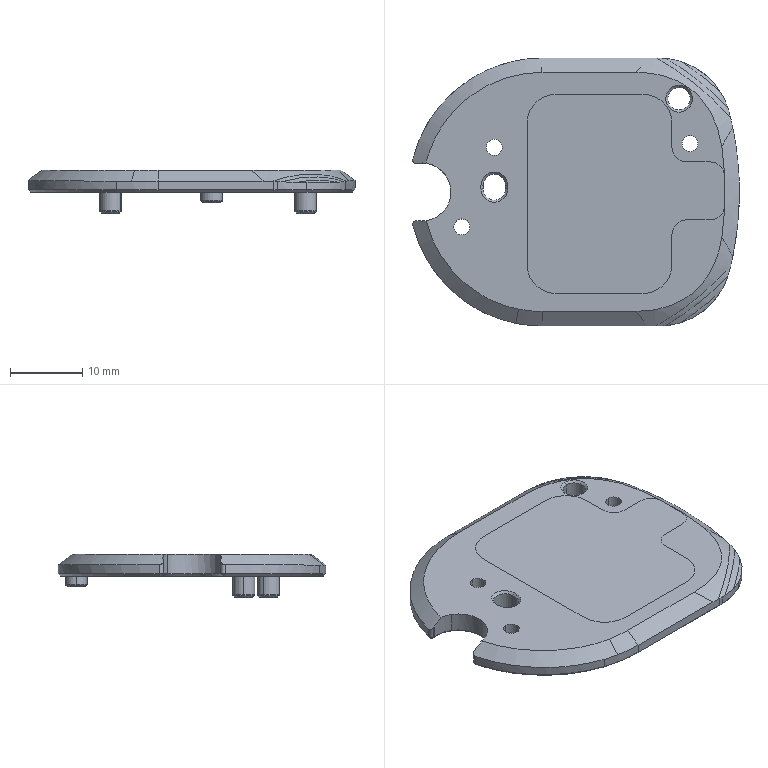NC program | NX | posted with a generic post | part box 45.101 x 36.973 x 6 mm
Lines 4825 to 5084 of 5084:
(PLANAR_MILL_COPY_COPY , TOOL : D6A45)
N9594 T01 M6
N9596 G54
N9598 G17 G0 G90 X-0.654 Y21.303 S9500 M3
N9600 G43 Z30. H1
N9602 Z-1.5
N9604 G94 G1 Z-4.5 F1250.
N9606 X-0.572 Y20.415
N9608 G3 X-0.145 Y19.685 R1.
N9610 G1 X4.605
N9612 G2 X23.698 Y4.829 R19.7
N9614 X21.748 Y2.738 R1.7
N9616 G3 X21.748 Y-2.773 R-2.8
N9618 G2 X23.697 Y-4.864 R1.7
N9620 X10.779 Y-18.722 R19.7
N9622 X7.772 Y-19.444 R19.699
N9624 X4.69 Y-19.686 R19.701
N9626 G1 X-11.31 Y-19.685
N9628 G2 X-11.562 Y-19.683 R19.698
N9630 X-11.814 Y-19.678 R19.699
N9632 X-16.395 Y-18.568 R11.2
N9634 X-22.306 Y-11.325 R11.2
N9636 X-22.304 Y11.3 R45.001
N9638 X-11.747 Y19.68 R11.2
N9640 X-11.247 Y19.686 R19.699
N9642 G1 X-5.267
N9644 G3 X-4.84 Y20.415 R1.
N9646 G1 X-4.757 Y21.303
N9648 Z-1.5
N9650 G0 Z30.
(PLANAR_MILL_COPY_COPY_COPY , TOOL : D6A45)
N9652 X-16.558 Y6.929
N9654 Z-1.
N9656 G1 X-16.576 Y6.442 Z-1.132
N9658 X-16.348 Y6.048 Z-1.254
N9660 X-15.954 Y5.82 Z-1.376
N9662 X-15.498 Z-1.498
N9664 X-15.104 Y6.048 Z-1.62
N9666 X-14.876 Y6.442 Z-1.742
N9668 Y6.898 Z-1.864
N9670 X-15.104 Y7.292 Z-1.986
N9672 X-15.498 Y7.52 Z-2.108
N9674 X-15.954 Z-2.23
N9676 X-16.348 Y7.292 Z-2.352
N9678 X-16.576 Y6.898 Z-2.474
N9680 Y6.442 Z-2.596
N9682 X-16.348 Y6.048 Z-2.718
N9684 X-15.954 Y5.82 Z-2.84
N9686 X-15.498 Z-2.963
N9688 X-15.104 Y6.048 Z-3.085
N9690 X-14.876 Y6.442 Z-3.207
N9692 Y6.898 Z-3.329
N9694 X-15.104 Y7.292 Z-3.451
N9696 X-15.498 Y7.52 Z-3.573
N9698 X-15.954 Z-3.695
N9700 X-16.348 Y7.292 Z-3.817
N9702 X-16.576 Y6.898 Z-3.939
N9704 Y6.67 Z-4.
N9706 G3 X-15.726 Y5.82 R0.85
N9708 X-16.576 Y6.67 R-0.85
N9710 X-16.397 Y6.287 R0.5
N9712 G1 Z-1.
N9714 G0 Z30.
N9716 X-14.764 Y12.485
N9718 Z-1.
N9720 G1 X-14.707 Y12.389 Z-1.03
N9722 X-14.426 Y12.22 Z-1.118
N9724 X-14.026 Z-1.225
N9726 X-13.745 Y12.389 Z-1.313
N9728 X-13.576 Y12.67 Z-1.401
N9730 Y13.07 Z-1.508
N9732 X-13.745 Y13.351 Z-1.596
N9734 X-14.026 Y13.52 Z-1.684
N9736 X-14.426 Z-1.791
N9738 X-14.707 Y13.351 Z-1.879
N9740 X-14.876 Y13.07 Z-1.967
N9742 Y12.67 Z-2.074
N9744 X-14.707 Y12.389 Z-2.161
N9746 X-14.426 Y12.22 Z-2.249
N9748 X-14.026 Z-2.356
N9750 X-13.745 Y12.389 Z-2.444
N9752 X-13.576 Y12.67 Z-2.532
N9754 Y13.07 Z-2.639
N9756 X-13.745 Y13.351 Z-2.727
N9758 X-14.026 Y13.52 Z-2.815
N9760 X-14.426 Z-2.922
N9762 X-14.707 Y13.351 Z-3.01
N9764 X-14.876 Y13.07 Z-3.098
N9766 Y12.67 Z-3.205
N9768 X-14.707 Y12.389 Z-3.293
N9770 X-14.426 Y12.22 Z-3.381
N9772 X-14.026 Z-3.488
N9774 X-13.745 Y12.389 Z-3.576
N9776 X-13.576 Y12.67 Z-3.664
N9778 Y13.07 Z-3.771
N9780 X-13.745 Y13.351 Z-3.859
N9782 X-14.026 Y13.52 Z-3.946
N9784 X-14.226 Z-4.
N9786 G3 X-14.876 Y12.87 R0.65
N9788 X-14.226 Y13.52 R-0.65
N9790 X-14.609 Y13.341 R0.5
N9792 G1 Z-1.
N9794 G0 Z30.
N9796 X12.106 Y5.911
N9798 Z-1.
N9800 G1 X12.124 Y6.398 Z-1.132
N9802 X11.896 Y6.792 Z-1.254
N9804 X11.502 Y7.02 Z-1.376
N9806 X11.046 Z-1.498
N9808 X10.652 Y6.792 Z-1.62
N9810 X10.424 Y6.398 Z-1.742
N9812 Y5.942 Z-1.864
N9814 X10.652 Y5.548 Z-1.986
N9816 X11.046 Y5.32 Z-2.108
N9818 X11.502 Z-2.23
N9820 X11.896 Y5.548 Z-2.352
N9822 X12.124 Y5.942 Z-2.474
N9824 Y6.398 Z-2.596
N9826 X11.896 Y6.792 Z-2.718
N9828 X11.502 Y7.02 Z-2.84
N9830 X11.046 Z-2.963
N9832 X10.652 Y6.792 Z-3.085
N9834 X10.424 Y6.398 Z-3.207
N9836 Y5.942 Z-3.329
N9838 X10.652 Y5.548 Z-3.451
N9840 X11.046 Y5.32 Z-3.573
N9842 X11.502 Z-3.695
N9844 X11.896 Y5.548 Z-3.817
N9846 X12.124 Y5.942 Z-3.939
N9848 Y6.17 Z-4.
N9850 G3 X11.274 Y7.02 R0.85
N9852 X12.124 Y6.17 R-0.85
N9854 X11.946 Y6.553 R0.5
N9856 G1 Z-1.
N9858 G0 Z30.
N9860 X11.769 Y-0.038
N9862 Z-1.
N9864 G1 X11.924 Y0.22 Z-1.081
N9866 Y1.12 Z-1.322
N9868 X11.755 Y1.401 Z-1.41
N9870 X11.474 Y1.57 Z-1.498
N9872 X11.074 Z-1.605
N9874 X10.793 Y1.401 Z-1.693
N9876 X10.624 Y1.12 Z-1.78
N9878 Y0.22 Z-2.021
N9880 X10.793 Y-0.061 Z-2.109
N9882 X11.074 Y-0.23 Z-2.197
N9884 X11.474 Z-2.304
N9886 X11.755 Y-0.061 Z-2.392
N9888 X11.924 Y0.22 Z-2.48
N9890 Y1.12 Z-2.721
N9892 X11.755 Y1.401 Z-2.809
N9894 X11.474 Y1.57 Z-2.897
N9896 X11.074 Z-3.004
N9898 X10.793 Y1.401 Z-3.092
N9900 X10.624 Y1.12 Z-3.18
N9902 Y0.22 Z-3.421
N9904 X10.793 Y-0.061 Z-3.509
N9906 X11.074 Y-0.23 Z-3.597
N9908 X11.474 Z-3.704
N9910 X11.755 Y-0.061 Z-3.792
N9912 X11.924 Y0.22 Z-3.879
N9914 Y0.67 Z-4.
N9916 Y0.92
N9918 G3 X11.274 Y1.57 R0.65
N9920 X10.624 Y0.92 R0.65
N9922 G1 Y0.42
N9924 G3 X11.274 Y-0.23 R0.65
N9926 X11.924 Y0.42 R0.65
N9928 G1 Y0.67
N9930 G3 X11.567 Y1.436 R1.
N9932 G1 Z-1.
N9934 G0 Z30.
N9936 X15.515 Y-5.662
N9938 Z-1.
N9940 G1 X16.002 Y-5.68 Z-1.132
N9942 X16.396 Y-5.452 Z-1.254
N9944 X16.624 Y-5.058 Z-1.376
N9946 Y-4.602 Z-1.498
N9948 X16.396 Y-4.208 Z-1.62
N9950 X16.002 Y-3.98 Z-1.742
N9952 X15.546 Z-1.864
N9954 X15.152 Y-4.208 Z-1.986
N9956 X14.924 Y-4.602 Z-2.108
N9958 Y-5.058 Z-2.23
N9960 X15.152 Y-5.452 Z-2.352
N9962 X15.546 Y-5.68 Z-2.474
N9964 X16.002 Z-2.596
N9966 X16.396 Y-5.452 Z-2.718
N9968 X16.624 Y-5.058 Z-2.84
N9970 Y-4.602 Z-2.963
N9972 X16.396 Y-4.208 Z-3.085
N9974 X16.002 Y-3.98 Z-3.207
N9976 X15.546 Z-3.329
N9978 X15.152 Y-4.208 Z-3.451
N9980 X14.924 Y-4.602 Z-3.573
N9982 Y-5.058 Z-3.695
N9984 X15.152 Y-5.452 Z-3.817
N9986 X15.546 Y-5.68 Z-3.939
N9988 X15.774 Z-4.
N9990 G3 X16.624 Y-4.83 R0.85
N9992 X15.774 Y-5.68 R-0.85
N9994 X16.157 Y-5.501 R0.5
N9996 G1 Z-1.
N9998 G0 Z30.
N10000 M5
(刀补11 , TOOL : D4)
N10002 T11 M6
N10004 G54
N10006 G17 G0 G90 X-20.217 Y-8.135 S9500 M3
N10008 G43 Z30. H11
N10010 Z-2.
N10012 G94 G1 Z-3. F1250.
N10014 G41 X-20.131 Y-8.085 D11
N10016 X-19.372 Y-7.449
N10018 G3 X-19.23 Y-7.142 R0.4
N10020 G2 X-15.679 Y-3.592 R3.55
N10022 X-19.23 Y-7.142 R-3.55
N10024 G3 X-19.372 Y-6.836 R0.4
N10026 G1 X-20.131 Y-6.2
N10028 G40
N10030 X-20.217 Y-6.15
N10032 Z-2.
N10034 G0 Z30.
N10036 X12.241 Y-15.082
N10038 Z-2.
N10040 G1 Z-3.
N10042 G41 X12.191 Y-14.995
N10044 X11.555 Y-14.237
N10046 G3 X11.248 Y-14.094 R0.4
N10048 G2 X7.698 Y-10.544 R3.55
N10050 X11.248 Y-14.094 R-3.55
N10052 G3 X10.942 Y-14.237 R0.4
N10054 G1 X10.306 Y-14.995
N10056 G40
N10058 X10.256 Y-15.082
N10060 Z-2.
N10062 G0 Z30.
N10064 X-3.699 Y20.523
N10066 Z-2.
N10068 G1 Z-3.
N10070 G41 X-3.649 Y20.436
N10072 X-3.013 Y19.678
N10074 G3 X-2.707 Y19.535 R0.4
N10076 G2 X0.843 Y15.985 R3.55
N10078 X-2.707 Y19.535 R-3.55
N10080 G3 X-2.4 Y19.678 R0.4
N10082 G1 X-1.764 Y20.436
N10084 G40
N10086 X-1.714 Y20.523
N10088 Z-2.
N10090 G0 Z30.
N10092 M5
N10094 M2